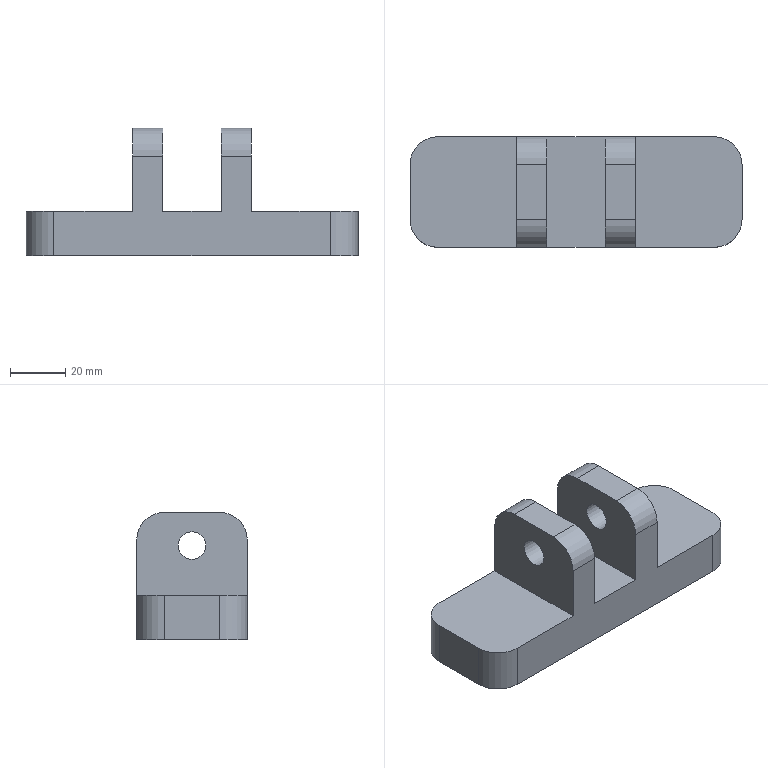NC program | NX | posted with a generic post | part box 120 x 40 x 46 mm
Lines 17839 to 19901 of 19901:
(FLOOR_FACING , TOOL : D16精光)
N35664 T03 M6
N35666 G53
N35668 G17 G0 G90 X-2.397 Y-31.1 S2200 M3
N35670 G43 Z20. H3
N35672 Z-27.
N35674 G94 G1 Z-30. F600.
N35676 Y-28.
N35678 Y28.
N35680 X2.4
N35682 Y-28.
N35684 Y-31.1
N35686 Z-27.
N35688 G0 Z20.
N35690 X56. Y30.125
N35692 Z-27.
N35694 G1 Z-30.
N35696 Y26.971
N35698 Y-26.971
N35700 G2 X50. Y-28. R18.
N35702 G1 X47.2
N35704 Y28.
N35706 X38.4
N35708 Y-28.
N35710 X29.6
N35712 Y28.
N35714 Y31.1
N35716 Z-27.
N35718 G0 Z20.
N35720 X-56. Y-30.125
N35722 Z-27.
N35724 G1 Z-30.
N35726 Y-26.971
N35728 Y26.971
N35730 G2 X-50. Y28. R18.
N35732 G1 X-47.2
N35734 Y-28.
N35736 X-38.4
N35738 Y28.
N35740 X-29.6
N35742 Y-28.
N35744 Y-31.1
N35746 Z-27.
N35748 G0 Z20.
(PLANAR_MILL_1_COPY , TOOL : D16精光)
N35750 X-29.674 Y-30.985
N35752 Z-27.99
N35754 G1 Z-29.99
N35756 G41 X-29.5 Y-30. D3
N35758 Y-20.
N35760 Y20.
N35762 Y30.
N35764 G40
N35766 X-29.674 Y30.985
N35768 Z-27.99
N35770 G0 Z20.
N35772 Y-30.985
N35774 Z-27.99
N35776 G1 Z-29.99
N35778 G41 X-29.5 Y-30.
N35780 Y-20.
N35782 Y20.
N35784 Y30.
N35786 G40
N35788 X-29.674 Y30.985
N35790 Z-27.99
N35792 G0 Z20.
N35794 X-2.326
N35796 Z-27.99
N35798 G1 Z-29.99
N35800 G41 X-2.5 Y30.
N35802 Y20.
N35804 Y-20.
N35806 Y-30.
N35808 G40
N35810 X-2.326 Y-30.985
N35812 Z-27.99
N35814 G0 Z20.
N35816 Y30.985
N35818 Z-27.99
N35820 G1 Z-29.99
N35822 G41 X-2.5 Y30.
N35824 Y20.
N35826 Y-20.
N35828 Y-30.
N35830 G40
N35832 X-2.326 Y-30.985
N35834 Z-27.99
N35836 G0 Z20.
N35838 X2.326
N35840 Z-27.99
N35842 G1 Z-29.99
N35844 G41 X2.5 Y-30.
N35846 Y-20.
N35848 Y20.
N35850 Y30.
N35852 G40
N35854 X2.326 Y30.985
N35856 Z-27.99
N35858 G0 Z20.
N35860 Y-30.985
N35862 Z-27.99
N35864 G1 Z-29.99
N35866 G41 X2.5 Y-30.
N35868 Y-20.
N35870 Y20.
N35872 Y30.
N35874 G40
N35876 X2.326 Y30.985
N35878 Z-27.99
N35880 G0 Z20.
N35882 X29.674
N35884 Z-27.99
N35886 G1 Z-29.99
N35888 G41 X29.5 Y30.
N35890 Y20.
N35892 Y-20.
N35894 Y-30.
N35896 G40
N35898 X29.674 Y-30.985
N35900 Z-27.99
N35902 G0 Z20.
N35904 Y30.985
N35906 Z-27.99
N35908 G1 Z-29.99
N35910 G41 X29.5 Y30.
N35912 Y20.
N35914 Y-20.
N35916 Y-30.
N35918 G40
N35920 X29.674 Y-30.985
N35922 Z-27.99
N35924 G0 Z20.
(PLANAR_MILL_1 , TOOL : D16精光)
N35926 X51.826
N35928 Z-45.
N35930 G1 Z-47.
N35932 G41 X52. Y-30.
N35934 G3 X50. Y-28. R2.
N35936 G1 X-50.
N35938 G2 X-68. Y-10. R18.
N35940 G1 Y10.
N35942 G2 X-50. Y28. R18.
N35944 G1 X50.
N35946 G2 X68. Y10. R18.
N35948 G1 Y-10.
N35950 G2 X50. Y-28. R18.
N35952 G3 X48. Y-30. R2.
N35954 G40
N35956 G1 X48.174 Y-30.985
N35958 X51.826
N35960 G41 X52. Y-30.
N35962 G3 X50. Y-28. R2.
N35964 G1 X-50.
N35966 G2 X-68. Y-10. R18.
N35968 G1 Y10.
N35970 G2 X-50. Y28. R18.
N35972 G1 X50.
N35974 G2 X68. Y10. R18.
N35976 G1 Y-10.
N35978 G2 X50. Y-28. R18.
N35980 G3 X48. Y-30. R2.
N35982 G40
N35984 G1 X48.174 Y-30.985
N35986 Z-45.
N35988 G0 Z20.
N35990 M5
(ZLEVEL_PROFILE_STEEP , TOOL : D6R0.5)
N35992 T04 M6
N35994 G53
N35996 G17 G0 G90 X23.3 Y-16.205 S3000 M3
N35998 G43 Z20. H4
N36000 Z0.95
N36002 G94 G1 Z-0.05 F1500.
N36004 Y-15.323
N36006 G3 X21.5 Y-13.523 R1.8
N36008 G1 X10.5
N36010 Y-13.726 Z-0.075
N36012 Y-13.946 Z-0.1
N36014 X21.5
N36016 Y-14.102 Z-0.125
N36018 Y-14.268 Z-0.15
N36020 X10.5
N36022 Y-14.4 Z-0.175
N36024 Y-14.54 Z-0.2
N36026 X21.5
N36028 Y-14.656 Z-0.225
N36030 Y-14.778 Z-0.25
N36032 X10.5
N36034 Y-14.882 Z-0.275
N36036 Y-14.992 Z-0.3
N36038 X21.5
N36040 Y-15.088 Z-0.325
N36042 Y-15.188 Z-0.35
N36044 X10.5
N36046 Y-15.277 Z-0.375
N36048 Y-15.371 Z-0.4
N36050 X21.5
N36052 Y-15.454 Z-0.425
N36054 Y-15.541 Z-0.45
N36056 X10.5
N36058 Y-15.702 Z-0.5
N36060 X21.5
N36062 Y-15.854 Z-0.55
N36064 X10.5
N36066 Y-15.999 Z-0.6
N36068 X21.5
N36070 Y-16.137 Z-0.65
N36072 X10.5
N36074 Y-16.27 Z-0.7
N36076 X21.5
N36078 Y-16.397 Z-0.75
N36080 X10.5
N36082 Y-16.52 Z-0.8
N36084 X21.5
N36086 Y-16.639 Z-0.85
N36088 X10.5
N36090 Y-16.753 Z-0.9
N36092 X21.5
N36094 Y-16.864 Z-0.95
N36096 X10.5
N36098 Y-16.972 Z-1.
N36100 X21.5
N36102 Y-17.077 Z-1.05
N36104 X10.5
N36106 Y-17.179 Z-1.1
N36108 X21.5
N36110 Y-17.278 Z-1.15
N36112 X10.5
N36114 Y-17.374 Z-1.2
N36116 X21.5
N36118 Y-17.469 Z-1.25
N36120 X10.5
N36122 Y-17.561 Z-1.3
N36124 X21.5
N36126 Y-17.65 Z-1.35
N36128 X10.5
N36130 Y-17.738 Z-1.4
N36132 X21.5
N36134 Y-17.824 Z-1.45
N36136 X10.5
N36138 Y-17.908 Z-1.5
N36140 X21.5
N36142 Y-17.991 Z-1.55
N36144 X10.5
N36146 Y-18.071 Z-1.6
N36148 X21.5
N36150 Y-18.15 Z-1.65
N36152 X10.5
N36154 Y-18.228 Z-1.7
N36156 X21.5
N36158 Y-18.304 Z-1.75
N36160 X10.5
N36162 Y-18.379 Z-1.8
N36164 X21.5
N36166 Y-18.452 Z-1.85
N36168 X10.5
N36170 Y-18.524 Z-1.9
N36172 X21.5
N36174 Y-18.595 Z-1.95
N36176 X10.5
N36178 Y-18.664 Z-2.
N36180 X21.5
N36182 Y-18.733 Z-2.05
N36184 X10.5
N36186 Y-18.8 Z-2.1
N36188 X21.5
N36190 Y-18.866 Z-2.15
N36192 X10.5
N36194 Y-18.931 Z-2.2
N36196 X21.5
N36198 Y-18.995 Z-2.25
N36200 X10.5
N36202 Y-19.058 Z-2.3
N36204 X21.5
N36206 Y-19.12 Z-2.35
N36208 X10.5
N36210 Y-19.181 Z-2.4
N36212 X21.5
N36214 Y-19.241 Z-2.45
N36216 X10.5
N36218 Y-19.301 Z-2.5
N36220 X21.5
N36222 Y-19.359 Z-2.55
N36224 X10.5
N36226 Y-19.417 Z-2.6
N36228 X21.5
N36230 Y-19.473 Z-2.65
N36232 X10.5
N36234 Y-19.529 Z-2.7
N36236 X21.5
N36238 Y-19.584 Z-2.75
N36240 X10.5
N36242 Y-19.639 Z-2.8
N36244 X21.5
N36246 Y-19.692 Z-2.85
N36248 X10.5
N36250 Y-19.745 Z-2.9
N36252 X21.5
N36254 Y-19.797 Z-2.95
N36256 X10.5
N36258 Y-19.848 Z-3.
N36260 X21.5
N36262 Y-19.899 Z-3.05
N36264 X10.5
N36266 Y-19.949 Z-3.1
N36268 X21.5
N36270 Y-19.999 Z-3.15
N36272 X10.5
N36274 Y-20.047 Z-3.2
N36276 X21.5
N36278 Y-20.095 Z-3.25
N36280 X10.5
N36282 Y-20.143 Z-3.3
N36284 X21.5
N36286 Y-20.189 Z-3.35
N36288 X10.5
N36290 Y-20.236 Z-3.4
N36292 X21.5
N36294 Y-20.281 Z-3.45
N36296 X10.5
N36298 Y-20.326 Z-3.5
N36300 X21.5
N36302 Y-20.371 Z-3.55
N36304 X10.5
N36306 Y-20.415 Z-3.6
N36308 X21.5
N36310 Y-20.458 Z-3.65
N36312 X10.5
N36314 Y-20.501 Z-3.7
N36316 X21.5
N36318 Y-20.543 Z-3.75
N36320 X10.5
N36322 Y-20.585 Z-3.8
N36324 X21.5
N36326 Y-20.626 Z-3.85
N36328 X10.5
N36330 Y-20.666 Z-3.9
N36332 X21.5
N36334 Y-20.707 Z-3.95
N36336 X10.5
N36338 Y-20.746 Z-4.
N36340 X21.5
N36342 Y-20.785 Z-4.05
N36344 X10.5
N36346 Y-20.824 Z-4.1
N36348 X21.5
N36350 Y-20.862 Z-4.15
N36352 X10.5
N36354 Y-20.9 Z-4.2
N36356 X21.5
N36358 Y-20.937 Z-4.25
N36360 X10.5
N36362 Y-20.974 Z-4.3
N36364 X21.5
N36366 Y-21.01 Z-4.35
N36368 X10.5
N36370 Y-21.046 Z-4.4
N36372 X21.5
N36374 Y-21.082 Z-4.45
N36376 X10.5
N36378 Y-21.117 Z-4.5
N36380 X21.5
N36382 Y-21.151 Z-4.55
N36384 X10.5
N36386 Y-21.186 Z-4.6
N36388 X21.5
N36390 Y-21.219 Z-4.65
N36392 X10.5
N36394 Y-21.253 Z-4.7
N36396 X21.5
N36398 Y-21.286 Z-4.75
N36400 X10.5
N36402 Y-21.318 Z-4.8
N36404 X21.5
N36406 Y-21.35 Z-4.85
N36408 X10.5
N36410 Y-21.382 Z-4.9
N36412 X21.5
N36414 Y-21.413 Z-4.95
N36416 X10.5
N36418 Y-21.444 Z-5.
N36420 X21.5
N36422 Y-21.475 Z-5.05
N36424 X10.5
N36426 Y-21.505 Z-5.1
N36428 X21.5
N36430 Y-21.535 Z-5.15
N36432 X10.5
N36434 Y-21.564 Z-5.2
N36436 X21.5
N36438 Y-21.593 Z-5.25
N36440 X10.5
N36442 Y-21.622 Z-5.3
N36444 X21.5
N36446 Y-21.65 Z-5.35
N36448 X10.5
N36450 Y-21.678 Z-5.4
N36452 X21.5
N36454 Y-21.706 Z-5.45
N36456 X10.5
N36458 Y-21.733 Z-5.5
N36460 X21.5
N36462 Y-21.76 Z-5.55
N36464 X10.5
N36466 Y-21.787 Z-5.6
N36468 X21.5
N36470 Y-21.813 Z-5.65
N36472 X10.5
N36474 Y-21.839 Z-5.7
N36476 X21.5
N36478 Y-21.864 Z-5.75
N36480 X10.5
N36482 Y-21.889 Z-5.8
N36484 X21.5
N36486 Y-21.914 Z-5.85
N36488 X10.5
N36490 Y-21.939 Z-5.9
N36492 X21.5
N36494 Y-21.963 Z-5.95
N36496 X10.5
N36498 Y-21.987 Z-6.
N36500 X21.5
N36502 Y-22.01 Z-6.05
N36504 X10.5
N36506 Y-22.034 Z-6.1
N36508 X21.5
N36510 Y-22.057 Z-6.15
N36512 X10.5
N36514 Y-22.079 Z-6.2
N36516 X21.5
N36518 Y-22.101 Z-6.25
N36520 X10.5
N36522 Y-22.123 Z-6.3
N36524 X21.5
N36526 Y-22.145 Z-6.35
N36528 X10.5
N36530 Y-22.166 Z-6.4
N36532 X21.5
N36534 Y-22.187 Z-6.45
N36536 X10.5
N36538 Y-22.208 Z-6.5
N36540 X21.5
N36542 Y-22.229 Z-6.55
N36544 X10.5
N36546 Y-22.249 Z-6.6
N36548 X21.5
N36550 Y-22.269 Z-6.65
N36552 X10.5
N36554 Y-22.288 Z-6.7
N36556 X21.5
N36558 Y-22.308 Z-6.75
N36560 X10.5
N36562 Y-22.326 Z-6.8
N36564 X21.5
N36566 Y-22.345 Z-6.85
N36568 X10.5
N36570 Y-22.364 Z-6.9
N36572 X21.5
N36574 Y-22.382 Z-6.95
N36576 X10.5
N36578 Y-22.399 Z-7.
N36580 X21.5
N36582 Y-22.417 Z-7.05
N36584 X10.5
N36586 Y-22.434 Z-7.1
N36588 X21.5
N36590 Y-22.451 Z-7.15
N36592 X10.5
N36594 Y-22.468 Z-7.2
N36596 X21.5
N36598 Y-22.484 Z-7.25
N36600 X10.5
N36602 Y-22.501 Z-7.3
N36604 X21.5
N36606 Y-22.516 Z-7.35
N36608 X10.5
N36610 Y-22.532 Z-7.4
N36612 X21.5
N36614 Y-22.547 Z-7.45
N36616 X10.5
N36618 Y-22.562 Z-7.5
N36620 X21.5
N36622 Y-22.577 Z-7.55
N36624 X10.5
N36626 Y-22.592 Z-7.6
N36628 X21.5
N36630 Y-22.606 Z-7.65
N36632 X10.5
N36634 Y-22.62 Z-7.7
N36636 X21.5
N36638 Y-22.633 Z-7.75
N36640 X10.5
N36642 Y-22.647 Z-7.8
N36644 X21.5
N36646 Y-22.66 Z-7.85
N36648 X10.5
N36650 Y-22.673 Z-7.9
N36652 X21.5
N36654 Y-22.686 Z-7.95
N36656 X10.5
N36658 Y-22.698 Z-8.
N36660 X21.5
N36662 Y-22.71 Z-8.05
N36664 X10.5
N36666 Y-22.722 Z-8.1
N36668 X21.5
N36670 Y-22.734 Z-8.15
N36672 X10.5
N36674 Y-22.745 Z-8.2
N36676 X21.5
N36678 Y-22.756 Z-8.25
N36680 X10.5
N36682 Y-22.767 Z-8.3
N36684 X21.5
N36686 Y-22.778 Z-8.35
N36688 X10.5
N36690 Y-22.788 Z-8.4
N36692 X21.5
N36694 Y-22.798 Z-8.45
N36696 X10.5
N36698 Y-22.808 Z-8.5
N36700 X21.5
N36702 Y-22.817 Z-8.55
N36704 X10.5
N36706 Y-22.827 Z-8.6
N36708 X21.5
N36710 Y-22.836 Z-8.65
N36712 X10.5
N36714 Y-22.845 Z-8.7
N36716 X21.5
N36718 Y-22.853 Z-8.75
N36720 X10.5
N36722 Y-22.861 Z-8.8
N36724 X21.5
N36726 Y-22.87 Z-8.85
N36728 X10.5
N36730 Y-22.877 Z-8.9
N36732 X21.5
N36734 Y-22.885 Z-8.95
N36736 X10.5
N36738 Y-22.892 Z-9.
N36740 X21.5
N36742 Y-22.899 Z-9.05
N36744 X10.5
N36746 Y-22.906 Z-9.1
N36748 X21.5
N36750 Y-22.913 Z-9.15
N36752 X10.5
N36754 Y-22.919 Z-9.2
N36756 X21.5
N36758 Y-22.925 Z-9.25
N36760 X10.5
N36762 Y-22.931 Z-9.3
N36764 X21.5
N36766 Y-22.937 Z-9.35
N36768 X10.5
N36770 Y-22.942 Z-9.4
N36772 X21.5
N36774 Y-22.947 Z-9.45
N36776 X10.5
N36778 Y-22.952 Z-9.5
N36780 X21.5
N36782 Y-22.957 Z-9.55
N36784 X10.5
N36786 Y-22.961 Z-9.6
N36788 X21.5
N36790 Y-22.966 Z-9.65
N36792 X10.5
N36794 Y-22.969 Z-9.7
N36796 X21.5
N36798 Y-22.973 Z-9.75
N36800 X10.5
N36802 Y-22.977 Z-9.8
N36804 X21.5
N36806 Y-22.98 Z-9.85
N36808 X10.5
N36810 Y-22.983 Z-9.9
N36812 X21.5
N36814 Y-22.986 Z-9.95
N36816 X10.5
N36818 Y-22.988 Z-10.
N36820 X21.5
N36822 Y-22.99 Z-10.05
N36824 X10.5
N36826 Y-22.992 Z-10.1
N36828 X21.5
N36830 Y-22.994 Z-10.15
N36832 X10.5
N36834 Y-22.996 Z-10.2
N36836 X21.5
N36838 Y-22.997 Z-10.25
N36840 X10.5
N36842 Y-22.998 Z-10.3
N36844 X21.5
N36846 Y-22.999 Z-10.35
N36848 X10.5
N36850 X10.501 Y-22.998 Z-10.4
N36852 X21.502
N36854 Z-10.45
N36856 X10.501
N36858 Y-22.999 Z-10.5
N36860 X21.502
N36862 G2 X23.302 Y-24.799 R1.8
N36864 G1 Y-25.722
N36866 Z-9.5
N36868 G0 Z20.
N36870 X8.7 Y16.189
N36872 Z0.95
N36874 G1 Z-0.05
N36876 Y15.323
N36878 G3 X10.5 Y13.523 R1.8
N36880 G1 X21.5
N36882 Y13.726 Z-0.075
N36884 Y13.946 Z-0.1
N36886 X10.5
N36888 Y14.102 Z-0.125
N36890 Y14.268 Z-0.15
N36892 X21.5
N36894 Y14.4 Z-0.175
N36896 Y14.54 Z-0.2
N36898 X10.5
N36900 Y14.656 Z-0.225
N36902 Y14.778 Z-0.25
N36904 X21.5
N36906 Y14.882 Z-0.275
N36908 Y14.992 Z-0.3
N36910 X10.5
N36912 Y15.088 Z-0.325
N36914 Y15.188 Z-0.35
N36916 X21.5
N36918 Y15.277 Z-0.375
N36920 Y15.371 Z-0.4
N36922 X10.5
N36924 Y15.454 Z-0.425
N36926 Y15.541 Z-0.45
N36928 X21.5
N36930 Y15.702 Z-0.5
N36932 X10.5
N36934 Y15.854 Z-0.55
N36936 X21.5
N36938 Y15.999 Z-0.6
N36940 X10.5
N36942 Y16.137 Z-0.65
N36944 X21.5
N36946 Y16.27 Z-0.7
N36948 X10.5
N36950 Y16.397 Z-0.75
N36952 X21.5
N36954 Y16.52 Z-0.8
N36956 X10.5
N36958 Y16.639 Z-0.85
N36960 X21.5
N36962 Y16.753 Z-0.9
N36964 X10.5
N36966 Y16.864 Z-0.95
N36968 X21.5
N36970 Y16.972 Z-1.
N36972 X10.5
N36974 Y17.077 Z-1.05
N36976 X21.5
N36978 Y17.179 Z-1.1
N36980 X10.5
N36982 Y17.278 Z-1.15
N36984 X21.5
N36986 Y17.374 Z-1.2
N36988 X10.5
N36990 Y17.469 Z-1.25
N36992 X21.5
N36994 Y17.561 Z-1.3
N36996 X10.5
N36998 Y17.65 Z-1.35
N37000 X21.5
N37002 Y17.738 Z-1.4
N37004 X10.5
N37006 Y17.824 Z-1.45
N37008 X21.5
N37010 Y17.908 Z-1.5
N37012 X10.5
N37014 Y17.991 Z-1.55
N37016 X21.5
N37018 Y18.071 Z-1.6
N37020 X10.5
N37022 Y18.15 Z-1.65
N37024 X21.5
N37026 Y18.228 Z-1.7
N37028 X10.5
N37030 Y18.304 Z-1.75
N37032 X21.5
N37034 Y18.379 Z-1.8
N37036 X10.5
N37038 Y18.452 Z-1.85
N37040 X21.5
N37042 Y18.524 Z-1.9
N37044 X10.5
N37046 Y18.595 Z-1.95
N37048 X21.5
N37050 Y18.664 Z-2.
N37052 X10.5
N37054 Y18.733 Z-2.05
N37056 X21.5
N37058 Y18.8 Z-2.1
N37060 X10.5
N37062 Y18.866 Z-2.15
N37064 X21.5
N37066 Y18.931 Z-2.2
N37068 X10.5
N37070 Y18.995 Z-2.25
N37072 X21.5
N37074 Y19.058 Z-2.3
N37076 X10.5
N37078 Y19.12 Z-2.35
N37080 X21.5
N37082 Y19.181 Z-2.4
N37084 X10.5
N37086 Y19.241 Z-2.45
N37088 X21.5
N37090 Y19.301 Z-2.5
N37092 X10.5
N37094 Y19.359 Z-2.55
N37096 X21.5
N37098 Y19.417 Z-2.6
N37100 X10.5
N37102 Y19.473 Z-2.65
N37104 X21.5
N37106 Y19.529 Z-2.7
N37108 X10.5
N37110 Y19.584 Z-2.75
N37112 X21.5
N37114 Y19.639 Z-2.8
N37116 X10.5
N37118 Y19.692 Z-2.85
N37120 X21.5
N37122 Y19.745 Z-2.9
N37124 X10.5
N37126 Y19.797 Z-2.95
N37128 X21.5
N37130 Y19.848 Z-3.
N37132 X10.5
N37134 Y19.899 Z-3.05
N37136 X21.5
N37138 Y19.949 Z-3.1
N37140 X10.5
N37142 Y19.999 Z-3.15
N37144 X21.5
N37146 Y20.047 Z-3.2
N37148 X10.5
N37150 Y20.095 Z-3.25
N37152 X21.5
N37154 Y20.143 Z-3.3
N37156 X10.5
N37158 Y20.189 Z-3.35
N37160 X21.5
N37162 Y20.236 Z-3.4
N37164 X10.5
N37166 Y20.281 Z-3.45
N37168 X21.5
N37170 Y20.326 Z-3.5
N37172 X10.5
N37174 Y20.371 Z-3.55
N37176 X21.5
N37178 Y20.415 Z-3.6
N37180 X10.5
N37182 Y20.458 Z-3.65
N37184 X21.5
N37186 Y20.501 Z-3.7
N37188 X10.5
N37190 Y20.543 Z-3.75
N37192 X21.5
N37194 Y20.585 Z-3.8
N37196 X10.5
N37198 Y20.626 Z-3.85
N37200 X21.5
N37202 Y20.666 Z-3.9
N37204 X10.5
N37206 Y20.707 Z-3.95
N37208 X21.5
N37210 Y20.746 Z-4.
N37212 X10.5
N37214 Y20.785 Z-4.05
N37216 X21.5
N37218 Y20.824 Z-4.1
N37220 X10.5
N37222 Y20.862 Z-4.15
N37224 X21.5
N37226 Y20.9 Z-4.2
N37228 X10.5
N37230 Y20.937 Z-4.25
N37232 X21.5
N37234 Y20.974 Z-4.3
N37236 X10.5
N37238 Y21.01 Z-4.35
N37240 X21.5
N37242 Y21.046 Z-4.4
N37244 X10.5
N37246 Y21.082 Z-4.45
N37248 X21.5
N37250 Y21.117 Z-4.5
N37252 X10.5
N37254 Y21.151 Z-4.55
N37256 X21.5
N37258 Y21.186 Z-4.6
N37260 X10.5
N37262 Y21.219 Z-4.65
N37264 X21.5
N37266 Y21.253 Z-4.7
N37268 X10.5
N37270 Y21.286 Z-4.75
N37272 X21.5
N37274 Y21.318 Z-4.8
N37276 X10.5
N37278 Y21.35 Z-4.85
N37280 X21.5
N37282 Y21.382 Z-4.9
N37284 X10.5
N37286 Y21.413 Z-4.95
N37288 X21.5
N37290 Y21.444 Z-5.
N37292 X10.5
N37294 Y21.475 Z-5.05
N37296 X21.5
N37298 Y21.505 Z-5.1
N37300 X10.5
N37302 Y21.535 Z-5.15
N37304 X21.5
N37306 Y21.564 Z-5.2
N37308 X10.5
N37310 Y21.593 Z-5.25
N37312 X21.5
N37314 Y21.622 Z-5.3
N37316 X10.5
N37318 Y21.65 Z-5.35
N37320 X21.5
N37322 Y21.678 Z-5.4
N37324 X10.5
N37326 Y21.706 Z-5.45
N37328 X21.5
N37330 Y21.733 Z-5.5
N37332 X10.5
N37334 Y21.76 Z-5.55
N37336 X21.5
N37338 Y21.787 Z-5.6
N37340 X10.5
N37342 Y21.813 Z-5.65
N37344 X21.5
N37346 Y21.839 Z-5.7
N37348 X10.5
N37350 Y21.864 Z-5.75
N37352 X21.5
N37354 Y21.889 Z-5.8
N37356 X10.5
N37358 Y21.914 Z-5.85
N37360 X21.5
N37362 Y21.939 Z-5.9
N37364 X10.5
N37366 Y21.963 Z-5.95
N37368 X21.5
N37370 Y21.987 Z-6.
N37372 X10.5
N37374 Y22.01 Z-6.05
N37376 X21.5
N37378 Y22.034 Z-6.1
N37380 X10.5
N37382 Y22.057 Z-6.15
N37384 X21.5
N37386 Y22.079 Z-6.2
N37388 X10.5
N37390 Y22.101 Z-6.25
N37392 X21.5
N37394 Y22.123 Z-6.3
N37396 X10.5
N37398 Y22.145 Z-6.35
N37400 X21.5
N37402 Y22.166 Z-6.4
N37404 X10.5
N37406 Y22.187 Z-6.45
N37408 X21.5
N37410 Y22.208 Z-6.5
N37412 X10.5
N37414 Y22.229 Z-6.55
N37416 X21.5
N37418 Y22.249 Z-6.6
N37420 X10.5
N37422 Y22.269 Z-6.65
N37424 X21.5
N37426 Y22.288 Z-6.7
N37428 X10.5
N37430 Y22.308 Z-6.75
N37432 X21.5
N37434 Y22.326 Z-6.8
N37436 X10.5
N37438 Y22.345 Z-6.85
N37440 X21.5
N37442 Y22.364 Z-6.9
N37444 X10.5
N37446 Y22.382 Z-6.95
N37448 X21.5
N37450 Y22.399 Z-7.
N37452 X10.5
N37454 Y22.417 Z-7.05
N37456 X21.5
N37458 Y22.434 Z-7.1
N37460 X10.5
N37462 Y22.451 Z-7.15
N37464 X21.5
N37466 Y22.468 Z-7.2
N37468 X10.5
N37470 Y22.484 Z-7.25
N37472 X21.5
N37474 Y22.501 Z-7.3
N37476 X10.5
N37478 Y22.516 Z-7.35
N37480 X21.5
N37482 Y22.532 Z-7.4
N37484 X10.5
N37486 Y22.547 Z-7.45
N37488 X21.5
N37490 Y22.562 Z-7.5
N37492 X10.5
N37494 Y22.577 Z-7.55
N37496 X21.5
N37498 Y22.592 Z-7.6
N37500 X10.5
N37502 Y22.606 Z-7.65
N37504 X21.5
N37506 Y22.62 Z-7.7
N37508 X10.5
N37510 Y22.633 Z-7.75
N37512 X21.5
N37514 Y22.647 Z-7.8
N37516 X10.5
N37518 Y22.66 Z-7.85
N37520 X21.5
N37522 Y22.673 Z-7.9
N37524 X10.5
N37526 Y22.686 Z-7.95
N37528 X21.5
N37530 Y22.698 Z-8.
N37532 X10.5
N37534 Y22.71 Z-8.05
N37536 X21.5
N37538 Y22.722 Z-8.1
N37540 X10.5
N37542 Y22.734 Z-8.15
N37544 X21.5
N37546 Y22.745 Z-8.2
N37548 X10.5
N37550 Y22.756 Z-8.25
N37552 X21.5
N37554 Y22.767 Z-8.3
N37556 X10.5
N37558 Y22.778 Z-8.35
N37560 X21.5
N37562 Y22.788 Z-8.4
N37564 X10.5
N37566 Y22.798 Z-8.45
N37568 X21.5
N37570 Y22.808 Z-8.5
N37572 X10.5
N37574 Y22.817 Z-8.55
N37576 X21.5
N37578 Y22.827 Z-8.6
N37580 X10.5
N37582 Y22.836 Z-8.65
N37584 X21.5
N37586 Y22.845 Z-8.7
N37588 X10.5
N37590 Y22.853 Z-8.75
N37592 X21.5
N37594 Y22.861 Z-8.8
N37596 X10.5
N37598 Y22.87 Z-8.85
N37600 X21.5
N37602 Y22.877 Z-8.9
N37604 X10.5
N37606 Y22.885 Z-8.95
N37608 X21.5
N37610 Y22.892 Z-9.
N37612 X10.5
N37614 Y22.899 Z-9.05
N37616 X21.5
N37618 Y22.906 Z-9.1
N37620 X10.5
N37622 Y22.913 Z-9.15
N37624 X21.5
N37626 Y22.919 Z-9.2
N37628 X10.5
N37630 Y22.925 Z-9.25
N37632 X21.5
N37634 Y22.931 Z-9.3
N37636 X10.5
N37638 Y22.937 Z-9.35
N37640 X21.5
N37642 Y22.942 Z-9.4
N37644 X10.5
N37646 Y22.947 Z-9.45
N37648 X21.5
N37650 Y22.952 Z-9.5
N37652 X10.5
N37654 Y22.957 Z-9.55
N37656 X21.5
N37658 Y22.961 Z-9.6
N37660 X10.5
N37662 Y22.966 Z-9.65
N37664 X21.5
N37666 Y22.969 Z-9.7
N37668 X10.5
N37670 Y22.973 Z-9.75
N37672 X21.5
N37674 Y22.977 Z-9.8
N37676 X10.5
N37678 Y22.98 Z-9.85
N37680 X21.5
N37682 Y22.983 Z-9.9
N37684 X10.5
N37686 Y22.986 Z-9.95
N37688 X21.5
N37690 Y22.988 Z-10.
N37692 X10.5
N37694 Y22.99 Z-10.05
N37696 X21.5
N37698 Y22.992 Z-10.1
N37700 X10.5
N37702 Y22.994 Z-10.15
N37704 X21.5
N37706 Y22.996 Z-10.2
N37708 X10.5
N37710 Y22.997 Z-10.25
N37712 X21.5
N37714 Y22.998 Z-10.3
N37716 X10.5
N37718 Y22.999 Z-10.35
N37720 X21.5
N37722 X21.508 Y22.998 Z-10.4
N37724 X10.501
N37726 Z-10.45
N37728 X21.508
N37730 Y22.999 Z-10.5
N37732 X10.501
N37734 G2 X8.701 Y24.799 R1.8
N37736 G1 Y25.723
N37738 Z-9.5
N37740 G0 Z20.
N37742 X-8.7 Y-16.189
N37744 Z0.95
N37746 G1 Z-0.05
N37748 Y-15.323
N37750 G3 X-10.5 Y-13.523 R1.8
N37752 G1 X-21.5
N37754 Y-13.753 Z-0.075
N37756 Y-13.946 Z-0.1
N37758 X-10.5
N37760 Y-14.115 Z-0.125
N37762 Y-14.268 Z-0.15
N37764 X-21.5
N37766 Y-14.409 Z-0.175
N37768 Y-14.54 Z-0.2
N37770 X-10.5
N37772 Y-14.662 Z-0.225
N37774 Y-14.778 Z-0.25
N37776 X-21.5
N37778 Y-14.887 Z-0.275
N37780 Y-14.992 Z-0.3
N37782 X-10.5
N37784 Y-15.092 Z-0.325
N37786 Y-15.188 Z-0.35
N37788 X-21.5
N37790 Y-15.281 Z-0.375
N37792 Y-15.371 Z-0.4
N37794 X-10.5
N37796 Y-15.457 Z-0.425
N37798 Y-15.541 Z-0.45
N37800 X-21.5
N37802 Y-15.702 Z-0.5
N37804 X-10.5
N37806 Y-15.854 Z-0.55
N37808 X-21.5
N37810 Y-15.999 Z-0.6
N37812 X-10.5
N37814 Y-16.137 Z-0.65
N37816 X-21.5
N37818 Y-16.27 Z-0.7
N37820 X-10.5
N37822 Y-16.397 Z-0.75
N37824 X-21.5
N37826 Y-16.52 Z-0.8
N37828 X-10.5
N37830 Y-16.639 Z-0.85
N37832 X-21.5
N37834 Y-16.753 Z-0.9
N37836 X-10.5
N37838 Y-16.864 Z-0.95
N37840 X-21.5
N37842 Y-16.972 Z-1.
N37844 X-10.5
N37846 Y-17.077 Z-1.05
N37848 X-21.5
N37850 Y-17.179 Z-1.1
N37852 X-10.5
N37854 Y-17.278 Z-1.15
N37856 X-21.5
N37858 Y-17.374 Z-1.2
N37860 X-10.5
N37862 Y-17.469 Z-1.25
N37864 X-21.5
N37866 Y-17.561 Z-1.3
N37868 X-10.5
N37870 Y-17.65 Z-1.35
N37872 X-21.5
N37874 Y-17.738 Z-1.4
N37876 X-10.5
N37878 Y-17.824 Z-1.45
N37880 X-21.5
N37882 Y-17.908 Z-1.5
N37884 X-10.5
N37886 Y-17.991 Z-1.55
N37888 X-21.5
N37890 Y-18.071 Z-1.6
N37892 X-10.5
N37894 Y-18.15 Z-1.65
N37896 X-21.5
N37898 Y-18.228 Z-1.7
N37900 X-10.5
N37902 Y-18.304 Z-1.75
N37904 X-21.5
N37906 Y-18.379 Z-1.8
N37908 X-10.5
N37910 Y-18.452 Z-1.85
N37912 X-21.5
N37914 Y-18.524 Z-1.9
N37916 X-10.5
N37918 Y-18.595 Z-1.95
N37920 X-21.5
N37922 Y-18.664 Z-2.
N37924 X-10.5
N37926 Y-18.733 Z-2.05
N37928 X-21.5
N37930 Y-18.8 Z-2.1
N37932 X-10.5
N37934 Y-18.866 Z-2.15
N37936 X-21.5
N37938 Y-18.931 Z-2.2
N37940 X-10.5
N37942 Y-18.995 Z-2.25
N37944 X-21.5
N37946 Y-19.058 Z-2.3
N37948 X-10.5
N37950 Y-19.12 Z-2.35
N37952 X-21.5
N37954 Y-19.181 Z-2.4
N37956 X-10.5
N37958 Y-19.241 Z-2.45
N37960 X-21.5
N37962 Y-19.301 Z-2.5
N37964 X-10.5
N37966 Y-19.359 Z-2.55
N37968 X-21.5
N37970 Y-19.417 Z-2.6
N37972 X-10.5
N37974 Y-19.473 Z-2.65
N37976 X-21.5
N37978 Y-19.529 Z-2.7
N37980 X-10.5
N37982 Y-19.584 Z-2.75
N37984 X-21.5
N37986 Y-19.639 Z-2.8
N37988 X-10.5
N37990 Y-19.692 Z-2.85
N37992 X-21.5
N37994 Y-19.745 Z-2.9
N37996 X-10.5
N37998 Y-19.797 Z-2.95
N38000 X-21.5
N38002 Y-19.848 Z-3.
N38004 X-10.5
N38006 Y-19.899 Z-3.05
N38008 X-21.5
N38010 Y-19.949 Z-3.1
N38012 X-10.5
N38014 Y-19.999 Z-3.15
N38016 X-21.5
N38018 Y-20.047 Z-3.2
N38020 X-10.5
N38022 Y-20.095 Z-3.25
N38024 X-21.5
N38026 Y-20.143 Z-3.3
N38028 X-10.5
N38030 Y-20.189 Z-3.35
N38032 X-21.5
N38034 Y-20.236 Z-3.4
N38036 X-10.5
N38038 Y-20.281 Z-3.45
N38040 X-21.5
N38042 Y-20.326 Z-3.5
N38044 X-10.5
N38046 Y-20.371 Z-3.55
N38048 X-21.5
N38050 Y-20.415 Z-3.6
N38052 X-10.5
N38054 Y-20.458 Z-3.65
N38056 X-21.5
N38058 Y-20.501 Z-3.7
N38060 X-10.5
N38062 Y-20.543 Z-3.75
N38064 X-21.5
N38066 Y-20.585 Z-3.8
N38068 X-10.5
N38070 Y-20.626 Z-3.85
N38072 X-21.5
N38074 Y-20.666 Z-3.9
N38076 X-10.5
N38078 Y-20.707 Z-3.95
N38080 X-21.5
N38082 Y-20.746 Z-4.
N38084 X-10.5
N38086 Y-20.785 Z-4.05
N38088 X-21.5
N38090 Y-20.824 Z-4.1
N38092 X-10.5
N38094 Y-20.862 Z-4.15
N38096 X-21.5
N38098 Y-20.9 Z-4.2
N38100 X-10.5
N38102 Y-20.937 Z-4.25
N38104 X-21.5
N38106 Y-20.974 Z-4.3
N38108 X-10.5
N38110 Y-21.01 Z-4.35
N38112 X-21.5
N38114 Y-21.046 Z-4.4
N38116 X-10.5
N38118 Y-21.082 Z-4.45
N38120 X-21.5
N38122 Y-21.117 Z-4.5
N38124 X-10.5
N38126 Y-21.151 Z-4.55
N38128 X-21.5
N38130 Y-21.186 Z-4.6
N38132 X-10.5
N38134 Y-21.219 Z-4.65
N38136 X-21.5
N38138 Y-21.253 Z-4.7
N38140 X-10.5
N38142 Y-21.286 Z-4.75
N38144 X-21.5
N38146 Y-21.318 Z-4.8
N38148 X-10.5
N38150 Y-21.35 Z-4.85
N38152 X-21.5
N38154 Y-21.382 Z-4.9
N38156 X-10.5
N38158 Y-21.413 Z-4.95
N38160 X-21.5
N38162 Y-21.444 Z-5.
N38164 X-10.5
N38166 Y-21.475 Z-5.05
N38168 X-21.5
N38170 Y-21.505 Z-5.1
N38172 X-10.5
N38174 Y-21.535 Z-5.15
N38176 X-21.5
N38178 Y-21.564 Z-5.2
N38180 X-10.5
N38182 Y-21.593 Z-5.25
N38184 X-21.5
N38186 Y-21.622 Z-5.3
N38188 X-10.5
N38190 Y-21.65 Z-5.35
N38192 X-21.5
N38194 Y-21.678 Z-5.4
N38196 X-10.5
N38198 Y-21.706 Z-5.45
N38200 X-21.5
N38202 Y-21.733 Z-5.5
N38204 X-10.5
N38206 Y-21.76 Z-5.55
N38208 X-21.5
N38210 Y-21.787 Z-5.6
N38212 X-10.5
N38214 Y-21.813 Z-5.65
N38216 X-21.5
N38218 Y-21.839 Z-5.7
N38220 X-10.5
N38222 Y-21.864 Z-5.75
N38224 X-21.5
N38226 Y-21.889 Z-5.8
N38228 X-10.5
N38230 Y-21.914 Z-5.85
N38232 X-21.5
N38234 Y-21.939 Z-5.9
N38236 X-10.5
N38238 Y-21.963 Z-5.95
N38240 X-21.5
N38242 Y-21.987 Z-6.
N38244 X-10.5
N38246 Y-22.01 Z-6.05
N38248 X-21.5
N38250 Y-22.034 Z-6.1
N38252 X-10.5
N38254 Y-22.057 Z-6.15
N38256 X-21.5
N38258 Y-22.079 Z-6.2
N38260 X-10.5
N38262 Y-22.101 Z-6.25
N38264 X-21.5
N38266 Y-22.123 Z-6.3
N38268 X-10.5
N38270 Y-22.145 Z-6.35
N38272 X-21.5
N38274 Y-22.166 Z-6.4
N38276 X-10.5
N38278 Y-22.187 Z-6.45
N38280 X-21.5
N38282 Y-22.208 Z-6.5
N38284 X-10.5
N38286 Y-22.229 Z-6.55
N38288 X-21.5
N38290 Y-22.249 Z-6.6
N38292 X-10.5
N38294 Y-22.269 Z-6.65
N38296 X-21.5
N38298 Y-22.288 Z-6.7
N38300 X-10.5
N38302 Y-22.308 Z-6.75
N38304 X-21.5
N38306 Y-22.326 Z-6.8
N38308 X-10.5
N38310 Y-22.345 Z-6.85
N38312 X-21.5
N38314 Y-22.364 Z-6.9
N38316 X-10.5
N38318 Y-22.382 Z-6.95
N38320 X-21.5
N38322 Y-22.399 Z-7.
N38324 X-10.5
N38326 Y-22.417 Z-7.05
N38328 X-21.5
N38330 Y-22.434 Z-7.1
N38332 X-10.5
N38334 Y-22.451 Z-7.15
N38336 X-21.5
N38338 Y-22.468 Z-7.2
N38340 X-10.5
N38342 Y-22.484 Z-7.25
N38344 X-21.5
N38346 Y-22.501 Z-7.3
N38348 X-10.5
N38350 Y-22.516 Z-7.35
N38352 X-21.5
N38354 Y-22.532 Z-7.4
N38356 X-10.5
N38358 Y-22.547 Z-7.45
N38360 X-21.5
N38362 Y-22.562 Z-7.5
N38364 X-10.5
N38366 Y-22.577 Z-7.55
N38368 X-21.5
N38370 Y-22.592 Z-7.6
N38372 X-10.5
N38374 Y-22.606 Z-7.65
N38376 X-21.5
N38378 Y-22.62 Z-7.7
N38380 X-10.5
N38382 Y-22.633 Z-7.75
N38384 X-21.5
N38386 Y-22.647 Z-7.8
N38388 X-10.5
N38390 Y-22.66 Z-7.85
N38392 X-21.5
N38394 Y-22.673 Z-7.9
N38396 X-10.5
N38398 Y-22.686 Z-7.95
N38400 X-21.5
N38402 Y-22.698 Z-8.
N38404 X-10.5
N38406 Y-22.71 Z-8.05
N38408 X-21.5
N38410 Y-22.722 Z-8.1
N38412 X-10.5
N38414 Y-22.734 Z-8.15
N38416 X-21.5
N38418 Y-22.745 Z-8.2
N38420 X-10.5
N38422 Y-22.756 Z-8.25
N38424 X-21.5
N38426 Y-22.767 Z-8.3
N38428 X-10.5
N38430 Y-22.778 Z-8.35
N38432 X-21.5
N38434 Y-22.788 Z-8.4
N38436 X-10.5
N38438 Y-22.798 Z-8.45
N38440 X-21.5
N38442 Y-22.808 Z-8.5
N38444 X-10.5
N38446 Y-22.817 Z-8.55
N38448 X-21.5
N38450 Y-22.827 Z-8.6
N38452 X-10.5
N38454 Y-22.836 Z-8.65
N38456 X-21.5
N38458 Y-22.845 Z-8.7
N38460 X-10.5
N38462 Y-22.853 Z-8.75
N38464 X-21.5
N38466 Y-22.861 Z-8.8
N38468 X-10.5
N38470 Y-22.87 Z-8.85
N38472 X-21.5
N38474 Y-22.877 Z-8.9
N38476 X-10.5
N38478 Y-22.885 Z-8.95
N38480 X-21.5
N38482 Y-22.892 Z-9.
N38484 X-10.5
N38486 Y-22.899 Z-9.05
N38488 X-21.5
N38490 Y-22.906 Z-9.1
N38492 X-10.5
N38494 Y-22.913 Z-9.15
N38496 X-21.5
N38498 Y-22.919 Z-9.2
N38500 X-10.5
N38502 Y-22.925 Z-9.25
N38504 X-21.5
N38506 Y-22.931 Z-9.3
N38508 X-10.5
N38510 Y-22.937 Z-9.35
N38512 X-21.5
N38514 Y-22.942 Z-9.4
N38516 X-10.5
N38518 Y-22.947 Z-9.45
N38520 X-21.5
N38522 Y-22.952 Z-9.5
N38524 X-10.5
N38526 Y-22.957 Z-9.55
N38528 X-21.5
N38530 Y-22.961 Z-9.6
N38532 X-10.5
N38534 Y-22.966 Z-9.65
N38536 X-21.5
N38538 Y-22.969 Z-9.7
N38540 X-10.5
N38542 Y-22.973 Z-9.75
N38544 X-21.5
N38546 Y-22.977 Z-9.8
N38548 X-10.5
N38550 Y-22.98 Z-9.85
N38552 X-21.5
N38554 Y-22.983 Z-9.9
N38556 X-10.5
N38558 Y-22.986 Z-9.95
N38560 X-21.5
N38562 Y-22.988 Z-10.
N38564 X-10.5
N38566 Y-22.99 Z-10.05
N38568 X-21.5
N38570 Y-22.992 Z-10.1
N38572 X-10.5
N38574 Y-22.994 Z-10.15
N38576 X-21.5
N38578 Y-22.996 Z-10.2
N38580 X-10.5
N38582 Y-22.997 Z-10.25
N38584 X-21.5
N38586 Y-22.998 Z-10.3
N38588 X-10.5
N38590 Y-22.999 Z-10.35
N38592 X-21.5
N38594 X-21.508 Y-22.998 Z-10.4
N38596 X-10.501
N38598 Z-10.45
N38600 X-21.508
N38602 Y-22.999 Z-10.5
N38604 X-10.501
N38606 G2 X-8.701 Y-24.799 R1.8
N38608 G1 Y-25.723
N38610 Z-9.5
N38612 G0 Z20.
N38614 X-23.3 Y16.205
N38616 Z0.95
N38618 G1 Z-0.05
N38620 Y15.323
N38622 G3 X-21.5 Y13.523 R1.8
N38624 G1 X-10.5
N38626 Y13.753 Z-0.075
N38628 Y13.946 Z-0.1
N38630 X-21.5
N38632 Y14.115 Z-0.125
N38634 Y14.268 Z-0.15
N38636 X-10.5
N38638 Y14.409 Z-0.175
N38640 Y14.54 Z-0.2
N38642 X-21.5
N38644 Y14.662 Z-0.225
N38646 Y14.778 Z-0.25
N38648 X-10.5
N38650 Y14.887 Z-0.275
N38652 Y14.992 Z-0.3
N38654 X-21.5
N38656 Y15.092 Z-0.325
N38658 Y15.188 Z-0.35
N38660 X-10.5
N38662 Y15.281 Z-0.375
N38664 Y15.371 Z-0.4
N38666 X-21.5
N38668 Y15.457 Z-0.425
N38670 Y15.541 Z-0.45
N38672 X-10.5
N38674 Y15.702 Z-0.5
N38676 X-21.5
N38678 Y15.854 Z-0.55
N38680 X-10.5
N38682 Y15.999 Z-0.6
N38684 X-21.5
N38686 Y16.137 Z-0.65
N38688 X-10.5
N38690 Y16.27 Z-0.7
N38692 X-21.5
N38694 Y16.397 Z-0.75
N38696 X-10.5
N38698 Y16.52 Z-0.8
N38700 X-21.5
N38702 Y16.639 Z-0.85
N38704 X-10.5
N38706 Y16.753 Z-0.9
N38708 X-21.5
N38710 Y16.864 Z-0.95
N38712 X-10.5
N38714 Y16.972 Z-1.
N38716 X-21.5
N38718 Y17.077 Z-1.05
N38720 X-10.5
N38722 Y17.179 Z-1.1
N38724 X-21.5
N38726 Y17.278 Z-1.15
N38728 X-10.5
N38730 Y17.374 Z-1.2
N38732 X-21.5
N38734 Y17.469 Z-1.25
N38736 X-10.5
N38738 Y17.561 Z-1.3
N38740 X-21.5
N38742 Y17.65 Z-1.35
N38744 X-10.5
N38746 Y17.738 Z-1.4
N38748 X-21.5
N38750 Y17.824 Z-1.45
N38752 X-10.5
N38754 Y17.908 Z-1.5
N38756 X-21.5
N38758 Y17.991 Z-1.55
N38760 X-10.5
N38762 Y18.071 Z-1.6
N38764 X-21.5
N38766 Y18.15 Z-1.65
N38768 X-10.5
N38770 Y18.228 Z-1.7
N38772 X-21.5
N38774 Y18.304 Z-1.75
N38776 X-10.5
N38778 Y18.379 Z-1.8
N38780 X-21.5
N38782 Y18.452 Z-1.85
N38784 X-10.5
N38786 Y18.524 Z-1.9
N38788 X-21.5
N38790 Y18.595 Z-1.95
N38792 X-10.5
N38794 Y18.664 Z-2.
N38796 X-21.5
N38798 Y18.733 Z-2.05
N38800 X-10.5
N38802 Y18.8 Z-2.1
N38804 X-21.5
N38806 Y18.866 Z-2.15
N38808 X-10.5
N38810 Y18.931 Z-2.2
N38812 X-21.5
N38814 Y18.995 Z-2.25
N38816 X-10.5
N38818 Y19.058 Z-2.3
N38820 X-21.5
N38822 Y19.12 Z-2.35
N38824 X-10.5
N38826 Y19.181 Z-2.4
N38828 X-21.5
N38830 Y19.241 Z-2.45
N38832 X-10.5
N38834 Y19.301 Z-2.5
N38836 X-21.5
N38838 Y19.359 Z-2.55
N38840 X-10.5
N38842 Y19.417 Z-2.6
N38844 X-21.5
N38846 Y19.473 Z-2.65
N38848 X-10.5
N38850 Y19.529 Z-2.7
N38852 X-21.5
N38854 Y19.584 Z-2.75
N38856 X-10.5
N38858 Y19.639 Z-2.8
N38860 X-21.5
N38862 Y19.692 Z-2.85
N38864 X-10.5
N38866 Y19.745 Z-2.9
N38868 X-21.5
N38870 Y19.797 Z-2.95
N38872 X-10.5
N38874 Y19.848 Z-3.
N38876 X-21.5
N38878 Y19.899 Z-3.05
N38880 X-10.5
N38882 Y19.949 Z-3.1
N38884 X-21.5
N38886 Y19.999 Z-3.15
N38888 X-10.5
N38890 Y20.047 Z-3.2
N38892 X-21.5
N38894 Y20.095 Z-3.25
N38896 X-10.5
N38898 Y20.143 Z-3.3
N38900 X-21.5
N38902 Y20.189 Z-3.35
N38904 X-10.5
N38906 Y20.236 Z-3.4
N38908 X-21.5
N38910 Y20.281 Z-3.45
N38912 X-10.5
N38914 Y20.326 Z-3.5
N38916 X-21.5
N38918 Y20.371 Z-3.55
N38920 X-10.5
N38922 Y20.415 Z-3.6
N38924 X-21.5
N38926 Y20.458 Z-3.65
N38928 X-10.5
N38930 Y20.501 Z-3.7
N38932 X-21.5
N38934 Y20.543 Z-3.75
N38936 X-10.5
N38938 Y20.585 Z-3.8
N38940 X-21.5
N38942 Y20.626 Z-3.85
N38944 X-10.5
N38946 Y20.666 Z-3.9
N38948 X-21.5
N38950 Y20.707 Z-3.95
N38952 X-10.5
N38954 Y20.746 Z-4.
N38956 X-21.5
N38958 Y20.785 Z-4.05
N38960 X-10.5
N38962 Y20.824 Z-4.1
N38964 X-21.5
N38966 Y20.862 Z-4.15
N38968 X-10.5
N38970 Y20.9 Z-4.2
N38972 X-21.5
N38974 Y20.937 Z-4.25
N38976 X-10.5
N38978 Y20.974 Z-4.3
N38980 X-21.5
N38982 Y21.01 Z-4.35
N38984 X-10.5
N38986 Y21.046 Z-4.4
N38988 X-21.5
N38990 Y21.082 Z-4.45
N38992 X-10.5
N38994 Y21.117 Z-4.5
N38996 X-21.5
N38998 Y21.151 Z-4.55
N39000 X-10.5
N39002 Y21.186 Z-4.6
N39004 X-21.5
N39006 Y21.219 Z-4.65
N39008 X-10.5
N39010 Y21.253 Z-4.7
N39012 X-21.5
N39014 Y21.286 Z-4.75
N39016 X-10.5
N39018 Y21.318 Z-4.8
N39020 X-21.5
N39022 Y21.35 Z-4.85
N39024 X-10.5
N39026 Y21.382 Z-4.9
N39028 X-21.5
N39030 Y21.413 Z-4.95
N39032 X-10.5
N39034 Y21.444 Z-5.
N39036 X-21.5
N39038 Y21.475 Z-5.05
N39040 X-10.5
N39042 Y21.505 Z-5.1
N39044 X-21.5
N39046 Y21.535 Z-5.15
N39048 X-10.5
N39050 Y21.564 Z-5.2
N39052 X-21.5
N39054 Y21.593 Z-5.25
N39056 X-10.5
N39058 Y21.622 Z-5.3
N39060 X-21.5
N39062 Y21.65 Z-5.35
N39064 X-10.5
N39066 Y21.678 Z-5.4
N39068 X-21.5
N39070 Y21.706 Z-5.45
N39072 X-10.5
N39074 Y21.733 Z-5.5
N39076 X-21.5
N39078 Y21.76 Z-5.55
N39080 X-10.5
N39082 Y21.787 Z-5.6
N39084 X-21.5
N39086 Y21.813 Z-5.65
N39088 X-10.5
N39090 Y21.839 Z-5.7
N39092 X-21.5
N39094 Y21.864 Z-5.75
N39096 X-10.5
N39098 Y21.889 Z-5.8
N39100 X-21.5
N39102 Y21.914 Z-5.85
N39104 X-10.5
N39106 Y21.939 Z-5.9
N39108 X-21.5
N39110 Y21.963 Z-5.95
N39112 X-10.5
N39114 Y21.987 Z-6.
N39116 X-21.5
N39118 Y22.01 Z-6.05
N39120 X-10.5
N39122 Y22.034 Z-6.1
N39124 X-21.5
N39126 Y22.057 Z-6.15
N39128 X-10.5
N39130 Y22.079 Z-6.2
N39132 X-21.5
N39134 Y22.101 Z-6.25
N39136 X-10.5
N39138 Y22.123 Z-6.3
N39140 X-21.5
N39142 Y22.145 Z-6.35
N39144 X-10.5
N39146 Y22.166 Z-6.4
N39148 X-21.5
N39150 Y22.187 Z-6.45
N39152 X-10.5
N39154 Y22.208 Z-6.5
N39156 X-21.5
N39158 Y22.229 Z-6.55
N39160 X-10.5
N39162 Y22.249 Z-6.6
N39164 X-21.5
N39166 Y22.269 Z-6.65
N39168 X-10.5
N39170 Y22.288 Z-6.7
N39172 X-21.5
N39174 Y22.308 Z-6.75
N39176 X-10.5
N39178 Y22.326 Z-6.8
N39180 X-21.5
N39182 Y22.345 Z-6.85
N39184 X-10.5
N39186 Y22.364 Z-6.9
N39188 X-21.5
N39190 Y22.382 Z-6.95
N39192 X-10.5
N39194 Y22.399 Z-7.
N39196 X-21.5
N39198 Y22.417 Z-7.05
N39200 X-10.5
N39202 Y22.434 Z-7.1
N39204 X-21.5
N39206 Y22.451 Z-7.15
N39208 X-10.5
N39210 Y22.468 Z-7.2
N39212 X-21.5
N39214 Y22.484 Z-7.25
N39216 X-10.5
N39218 Y22.501 Z-7.3
N39220 X-21.5
N39222 Y22.516 Z-7.35
N39224 X-10.5
N39226 Y22.532 Z-7.4
N39228 X-21.5
N39230 Y22.547 Z-7.45
N39232 X-10.5
N39234 Y22.562 Z-7.5
N39236 X-21.5
N39238 Y22.577 Z-7.55
N39240 X-10.5
N39242 Y22.592 Z-7.6
N39244 X-21.5
N39246 Y22.606 Z-7.65
N39248 X-10.5
N39250 Y22.62 Z-7.7
N39252 X-21.5
N39254 Y22.633 Z-7.75
N39256 X-10.5
N39258 Y22.647 Z-7.8
N39260 X-21.5
N39262 Y22.66 Z-7.85
N39264 X-10.5
N39266 Y22.673 Z-7.9
N39268 X-21.5
N39270 Y22.686 Z-7.95
N39272 X-10.5
N39274 Y22.698 Z-8.
N39276 X-21.5
N39278 Y22.71 Z-8.05
N39280 X-10.5
N39282 Y22.722 Z-8.1
N39284 X-21.5
N39286 Y22.734 Z-8.15
N39288 X-10.5
N39290 Y22.745 Z-8.2
N39292 X-21.5
N39294 Y22.756 Z-8.25
N39296 X-10.5
N39298 Y22.767 Z-8.3
N39300 X-21.5
N39302 Y22.778 Z-8.35
N39304 X-10.5
N39306 Y22.788 Z-8.4
N39308 X-21.5
N39310 Y22.798 Z-8.45
N39312 X-10.5
N39314 Y22.808 Z-8.5
N39316 X-21.5
N39318 Y22.817 Z-8.55
N39320 X-10.5
N39322 Y22.827 Z-8.6
N39324 X-21.5
N39326 Y22.836 Z-8.65
N39328 X-10.5
N39330 Y22.845 Z-8.7
N39332 X-21.5
N39334 Y22.853 Z-8.75
N39336 X-10.5
N39338 Y22.861 Z-8.8
N39340 X-21.5
N39342 Y22.87 Z-8.85
N39344 X-10.5
N39346 Y22.877 Z-8.9
N39348 X-21.5
N39350 Y22.885 Z-8.95
N39352 X-10.5
N39354 Y22.892 Z-9.
N39356 X-21.5
N39358 Y22.899 Z-9.05
N39360 X-10.5
N39362 Y22.906 Z-9.1
N39364 X-21.5
N39366 Y22.913 Z-9.15
N39368 X-10.5
N39370 Y22.919 Z-9.2
N39372 X-21.5
N39374 Y22.925 Z-9.25
N39376 X-10.5
N39378 Y22.931 Z-9.3
N39380 X-21.5
N39382 Y22.937 Z-9.35
N39384 X-10.5
N39386 Y22.942 Z-9.4
N39388 X-21.5
N39390 Y22.947 Z-9.45
N39392 X-10.5
N39394 Y22.952 Z-9.5
N39396 X-21.5
N39398 Y22.957 Z-9.55
N39400 X-10.5
N39402 Y22.961 Z-9.6
N39404 X-21.5
N39406 Y22.966 Z-9.65
N39408 X-10.5
N39410 Y22.969 Z-9.7
N39412 X-21.5
N39414 Y22.973 Z-9.75
N39416 X-10.5
N39418 Y22.977 Z-9.8
N39420 X-21.5
N39422 Y22.98 Z-9.85
N39424 X-10.5
N39426 Y22.983 Z-9.9
N39428 X-21.5
N39430 Y22.986 Z-9.95
N39432 X-10.5
N39434 Y22.988 Z-10.
N39436 X-21.5
N39438 Y22.99 Z-10.05
N39440 X-10.5
N39442 Y22.992 Z-10.1
N39444 X-21.5
N39446 Y22.994 Z-10.15
N39448 X-10.5
N39450 Y22.996 Z-10.2
N39452 X-21.5
N39454 Y22.997 Z-10.25
N39456 X-10.5
N39458 Y22.998 Z-10.3
N39460 X-21.5
N39462 Y22.999 Z-10.35
N39464 X-10.5
N39466 X-10.501 Y22.998 Z-10.4
N39468 X-21.508
N39470 Z-10.45
N39472 X-10.501
N39474 Y22.999 Z-10.5
N39476 X-21.508
N39478 G2 X-23.308 Y24.799 R1.8
N39480 G1 Y25.721
N39482 Z-9.5
N39484 G0 Z20.
N39486 M5
(PLANAR_MILL_2 , TOOL : D6倒角刀)
N39488 T05 M6
N39490 G53
N39492 G17 G0 G90 X-23.5 Y-14. S3000 M3
N39494 G43 Z20. H5
N39496 Z0.
N39498 G94 G1 Z-2. F800.
N39500 Y-10.
N39502 Y10.
N39504 Y14.
N39506 Z0.
N39508 G0 Z20.
N39510 X-8.5
N39512 Z0.
N39514 G1 Z-2.
N39516 Y10.
N39518 Y-10.
N39520 Y-14.
N39522 Z0.
N39524 G0 Z20.
N39526 X8.5
N39528 Z0.
N39530 G1 Z-2.
N39532 Y-10.
N39534 Y10.
N39536 Y14.
N39538 Z0.
N39540 G0 Z20.
N39542 X23.5
N39544 Z0.
N39546 G1 Z-2.
N39548 Y10.
N39550 Y-10.
N39552 Y-14.
N39554 Z0.
N39556 G0 Z20.
(PLANAR_MILL_3 , TOOL : D6倒角刀)
N39558 X-22.6 Y-24.
N39560 Z-30.
N39562 G1 Z-32.
N39564 G3 X-24.6 Y-22. R2.
N39566 G1 X-50.
N39568 G2 X-62. Y-10. R12.
N39570 G1 Y10.
N39572 G2 X-50. Y22. R12.
N39574 G1 X-24.6
N39576 G3 X-22.6 Y24. R2.
N39578 G1 Z-30.
N39580 G0 Z20.
N39582 X-9.3
N39584 Z-30.
N39586 G1 Z-32.
N39588 G3 X-7.3 Y22. R2.
N39590 G1 X7.3
N39592 G3 X9.3 Y24. R2.
N39594 G1 Z-30.
N39596 G0 Z20.
N39598 X22.6
N39600 Z-30.
N39602 G1 Z-32.
N39604 G3 X24.6 Y22. R2.
N39606 G1 X50.
N39608 G2 X62. Y10. R12.
N39610 G1 Y-10.
N39612 G2 X50. Y-22. R12.
N39614 G1 X24.6
N39616 G3 X22.6 Y-24. R2.
N39618 G1 Z-30.
N39620 G0 Z20.
N39622 X9.3
N39624 Z-30.
N39626 G1 Z-32.
N39628 G3 X7.3 Y-22. R2.
N39630 G1 X-7.3
N39632 G3 X-9.3 Y-24. R2.
N39634 G1 Z-30.
N39636 G0 Z20.
N39638 M5
(PLANAR_MILL_4 , TOOL : D50面刀)
N39640 T01 M6
N39642 G54
N39644 G17 G0 G90 X100. Y0. S1600 M3
N39646 G43 Z20. H1
N39648 Z3.
N39650 G94 G1 Z0. F600.
N39652 X50.
N39654 X-50.
N39656 X-100.
N39658 Z3.
N39660 G0 Z20.
N39662 M5
(PLANAR_MILL_5 , TOOL : D6倒角刀)
N39664 T05 M6
N39666 G54
N39668 G17 G0 G90 X-2. Y24. S3000 M3
N39670 G43 Z20. H5
N39672 Z0.
N39674 G94 G1 Z-2. F600.
N39676 G3 X0. Y22. R2.
N39678 G1 X50.
N39680 G2 X62. Y10. R12.
N39682 G1 Y-10.
N39684 G2 X50. Y-22. R12.
N39686 G1 X-50.
N39688 G2 X-62. Y-10. R12.
N39690 G1 Y10.
N39692 G2 X-50. Y22. R12.
N39694 G1 X0.
N39696 G3 X2. Y24. R2.
N39698 G1 Z0.
N39700 G0 Z20.
(DRILLING , TOOL : D6倒角刀)
N39702 X34. Y0. S0
N39704 G81 G99 Z-40. F250. R-35.5
N39706 G80
N39708 G0 X34. Y0. Z20.
N39710 M5
(DRILLING_COPY , TOOL : D10钻头)
N39712 T10 M6
N39714 G54
N39716 G17 G0 G90 X34. Y0. S800 M3
N39718 G43 Z20. H10
N39720 G94 G83 G99 Z-53.5 F50. Q2. R-35.5
N39722 G80
N39724 G0 X34. Y0. Z20.
N39726 M5
N39728 M2